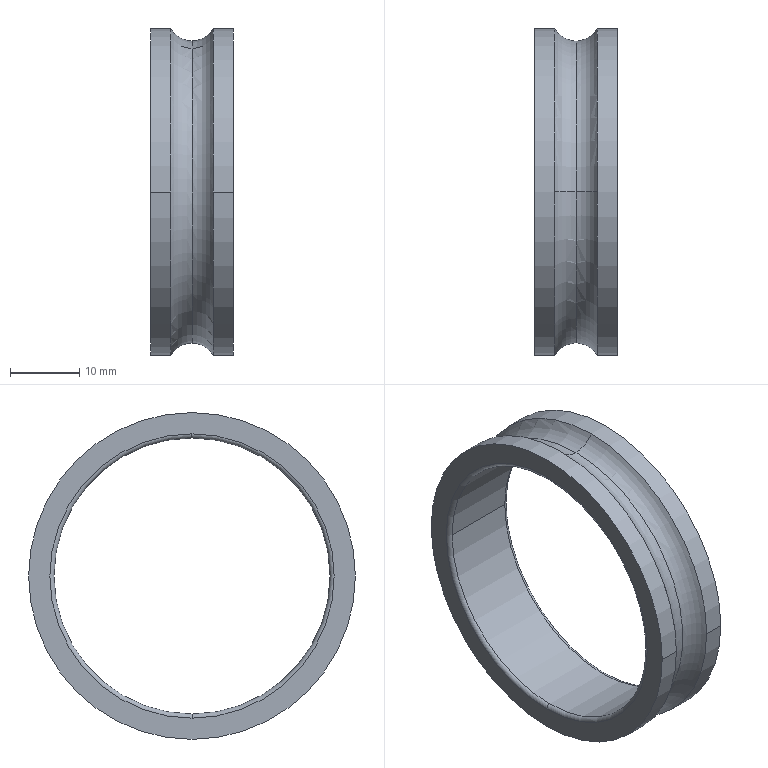Part | STEP file | bearing_6908_01V11 | 1 solid | 16 faces | box 12 x 47.33 x 47.33 mm | volume 4895 mm3 | torus 8 | cylinder 6 | plane 2 | commonest cylinder face diameters 47.33 x4 40 x2
STEP:
#1=CARTESIAN_POINT('',(0.,0.,0.));
#2=DIRECTION('',(0.,0.,1.));
#3=DIRECTION('',(1.,0.,0.));
#4=AXIS2_PLACEMENT_3D('',#1,#2,#3);
#5=CARTESIAN_POINT('',(3.099,0.,-23.665));
#6=VERTEX_POINT('',#5);
#7=CARTESIAN_POINT('',(3.099,23.665,0.));
#8=VERTEX_POINT('',#7);
#9=CARTESIAN_POINT('',(3.099,0.,0.));
#10=DIRECTION('',(1.,0.,0.));
#11=DIRECTION('',(0.,1.,0.));
#12=AXIS2_PLACEMENT_3D('',#9,#10,#11);
#13=CIRCLE('',#12,23.665);
#14=CARTESIAN_POINT('',(0.,0.,0.));
#15=DIRECTION('',(1.,0.,0.));
#16=DIRECTION('',(0.,0.,-1.));
#17=AXIS2_PLACEMENT_3D('',#14,#15,#16);
#18=TOROIDAL_SURFACE('',#17,25.497,3.6);
#19=CARTESIAN_POINT('',(-4.712,2.105));
#20=DIRECTION('',(1.,0.));
#21=VECTOR('',#20,1.);
#22=LINE('',#19,#21);
#23=(GEOMETRIC_REPRESENTATION_CONTEXT(2)PARAMETRIC_REPRESENTATION_CONTEXT()REPRESENTATION_CONTEXT('',''));
#24=DEFINITIONAL_REPRESENTATION('',(#22),#23);
#25=PCURVE('',#18,#24);
#26=CARTESIAN_POINT('',(4.549,0.,0.));
#27=DIRECTION('',(-1.,0.,0.));
#28=DIRECTION('',(0.,1.,0.));
#29=AXIS2_PLACEMENT_3D('',#26,#27,#28);
#30=CYLINDRICAL_SURFACE('',#29,23.665);
#31=CARTESIAN_POINT('',(6.283,1.451));
#32=DIRECTION('',(-1.,0.));
#33=VECTOR('',#32,1.);
#34=LINE('',#31,#33);
#35=(GEOMETRIC_REPRESENTATION_CONTEXT(2)PARAMETRIC_REPRESENTATION_CONTEXT()REPRESENTATION_CONTEXT('',''));
#36=DEFINITIONAL_REPRESENTATION('',(#34),#35);
#37=PCURVE('',#30,#36);
#38=SURFACE_CURVE('',#13,(#25,#37),.PCURVE_S1.);
#39=EDGE_CURVE('',#6,#8,#38,.T.);
#40=ORIENTED_EDGE('',*,*,#39,.T.);
#41=CARTESIAN_POINT('',(3.099,0.,23.665));
#42=VERTEX_POINT('',#41);
#43=CARTESIAN_POINT('',(3.099,0.,0.));
#44=DIRECTION('',(1.,0.,0.));
#45=DIRECTION('',(0.,1.,0.));
#46=AXIS2_PLACEMENT_3D('',#43,#44,#45);
#47=CIRCLE('',#46,23.665);
#48=CARTESIAN_POINT('',(1.571,2.105));
#49=DIRECTION('',(1.,0.));
#50=VECTOR('',#49,1.);
#51=LINE('',#48,#50);
#52=(GEOMETRIC_REPRESENTATION_CONTEXT(2)PARAMETRIC_REPRESENTATION_CONTEXT()REPRESENTATION_CONTEXT('',''));
#53=DEFINITIONAL_REPRESENTATION('',(#51),#52);
#54=PCURVE('',#18,#53);
#55=CARTESIAN_POINT('',(4.549,0.,0.));
#56=DIRECTION('',(-1.,0.,0.));
#57=DIRECTION('',(0.,1.,0.));
#58=AXIS2_PLACEMENT_3D('',#55,#56,#57);
#59=CYLINDRICAL_SURFACE('',#58,23.665);
#60=CARTESIAN_POINT('',(6.283,1.451));
#61=DIRECTION('',(-1.,0.));
#62=VECTOR('',#61,1.);
#63=LINE('',#60,#62);
#64=(GEOMETRIC_REPRESENTATION_CONTEXT(2)PARAMETRIC_REPRESENTATION_CONTEXT()REPRESENTATION_CONTEXT('',''));
#65=DEFINITIONAL_REPRESENTATION('',(#63),#64);
#66=PCURVE('',#59,#65);
#67=SURFACE_CURVE('',#47,(#54,#66),.PCURVE_S1.);
#68=EDGE_CURVE('',#8,#42,#67,.T.);
#69=ORIENTED_EDGE('',*,*,#68,.T.);
#70=CARTESIAN_POINT('',(0.,0.,21.898));
#71=VERTEX_POINT('',#70);
#72=CARTESIAN_POINT('',(0.,0.,25.497));
#73=DIRECTION('',(0.,1.,0.));
#74=DIRECTION('',(0.,0.,1.));
#75=AXIS2_PLACEMENT_3D('',#72,#73,#74);
#76=CIRCLE('',#75,3.6);
#77=CARTESIAN_POINT('',(3.142,0.));
#78=DIRECTION('',(0.,1.));
#79=VECTOR('',#78,1.);
#80=LINE('',#77,#79);
#81=(GEOMETRIC_REPRESENTATION_CONTEXT(2)PARAMETRIC_REPRESENTATION_CONTEXT()REPRESENTATION_CONTEXT('',''));
#82=DEFINITIONAL_REPRESENTATION('',(#80),#81);
#83=PCURVE('',#18,#82);
#84=CARTESIAN_POINT('',(0.,0.,0.));
#85=DIRECTION('',(1.,0.,0.));
#86=DIRECTION('',(0.,0.,-1.));
#87=AXIS2_PLACEMENT_3D('',#84,#85,#86);
#88=TOROIDAL_SURFACE('',#87,25.497,3.6);
#89=CARTESIAN_POINT('',(3.142,0.));
#90=DIRECTION('',(0.,1.));
#91=VECTOR('',#90,1.);
#92=LINE('',#89,#91);
#93=(GEOMETRIC_REPRESENTATION_CONTEXT(2)PARAMETRIC_REPRESENTATION_CONTEXT()REPRESENTATION_CONTEXT('',''));
#94=DEFINITIONAL_REPRESENTATION('',(#92),#93);
#95=PCURVE('',#88,#94);
#96=SURFACE_CURVE('',#76,(#83,#95),.PCURVE_S1.);
#97=EDGE_CURVE('',#42,#71,#96,.T.);
#98=ORIENTED_EDGE('',*,*,#97,.T.);
#99=CARTESIAN_POINT('',(0.,0.,-21.898));
#100=VERTEX_POINT('',#99);
#101=CARTESIAN_POINT('',(0.,0.,0.));
#102=DIRECTION('',(1.,0.,0.));
#103=DIRECTION('',(0.,0.,-1.));
#104=AXIS2_PLACEMENT_3D('',#101,#102,#103);
#105=CIRCLE('',#104,21.898);
#106=CARTESIAN_POINT('',(0.,3.142));
#107=DIRECTION('',(1.,0.));
#108=VECTOR('',#107,1.);
#109=LINE('',#106,#108);
#110=(GEOMETRIC_REPRESENTATION_CONTEXT(2)PARAMETRIC_REPRESENTATION_CONTEXT()REPRESENTATION_CONTEXT('',''));
#111=DEFINITIONAL_REPRESENTATION('',(#109),#110);
#112=PCURVE('',#18,#111);
#113=CARTESIAN_POINT('',(0.,0.,0.));
#114=DIRECTION('',(1.,0.,0.));
#115=DIRECTION('',(0.,0.,-1.));
#116=AXIS2_PLACEMENT_3D('',#113,#114,#115);
#117=TOROIDAL_SURFACE('',#116,25.497,3.6);
#118=CARTESIAN_POINT('',(0.,3.142));
#119=DIRECTION('',(1.,0.));
#120=VECTOR('',#119,1.);
#121=LINE('',#118,#120);
#122=(GEOMETRIC_REPRESENTATION_CONTEXT(2)PARAMETRIC_REPRESENTATION_CONTEXT()REPRESENTATION_CONTEXT('',''));
#123=DEFINITIONAL_REPRESENTATION('',(#121),#122);
#124=PCURVE('',#117,#123);
#125=SURFACE_CURVE('',#105,(#112,#124),.PCURVE_S1.);
#126=EDGE_CURVE('',#100,#71,#125,.T.);
#127=ORIENTED_EDGE('',*,*,#126,.F.);
#128=CARTESIAN_POINT('',(0.,0.,-25.497));
#129=DIRECTION('',(0.,-1.,0.));
#130=DIRECTION('',(0.,0.,-1.));
#131=AXIS2_PLACEMENT_3D('',#128,#129,#130);
#132=CIRCLE('',#131,3.6);
#133=CARTESIAN_POINT('',(0.,0.));
#134=DIRECTION('',(0.,1.));
#135=VECTOR('',#134,1.);
#136=LINE('',#133,#135);
#137=(GEOMETRIC_REPRESENTATION_CONTEXT(2)PARAMETRIC_REPRESENTATION_CONTEXT()REPRESENTATION_CONTEXT('',''));
#138=DEFINITIONAL_REPRESENTATION('',(#136),#137);
#139=PCURVE('',#18,#138);
#140=CARTESIAN_POINT('',(6.283,0.));
#141=DIRECTION('',(0.,1.));
#142=VECTOR('',#141,1.);
#143=LINE('',#140,#142);
#144=(GEOMETRIC_REPRESENTATION_CONTEXT(2)PARAMETRIC_REPRESENTATION_CONTEXT()REPRESENTATION_CONTEXT('',''));
#145=DEFINITIONAL_REPRESENTATION('',(#143),#144);
#146=PCURVE('',#88,#145);
#147=SURFACE_CURVE('',#132,(#139,#146),.PCURVE_S1.);
#148=EDGE_CURVE('',#6,#100,#147,.T.);
#149=ORIENTED_EDGE('',*,*,#148,.F.);
#150=EDGE_LOOP('',(#40,#69,#98,#127,#149));
#151=FACE_BOUND('',#150,.F.);
#152=ADVANCED_FACE('',(#151),#18,.F.);
#153=CARTESIAN_POINT('',(3.099,-23.665,0.));
#154=VERTEX_POINT('',#153);
#155=CARTESIAN_POINT('',(3.099,0.,0.));
#156=DIRECTION('',(1.,0.,0.));
#157=DIRECTION('',(0.,1.,0.));
#158=AXIS2_PLACEMENT_3D('',#155,#156,#157);
#159=CIRCLE('',#158,23.665);
#160=CARTESIAN_POINT('',(1.571,2.105));
#161=DIRECTION('',(1.,0.));
#162=VECTOR('',#161,1.);
#163=LINE('',#160,#162);
#164=(GEOMETRIC_REPRESENTATION_CONTEXT(2)PARAMETRIC_REPRESENTATION_CONTEXT()REPRESENTATION_CONTEXT('',''));
#165=DEFINITIONAL_REPRESENTATION('',(#163),#164);
#166=PCURVE('',#88,#165);
#167=CARTESIAN_POINT('',(6.283,1.451));
#168=DIRECTION('',(-1.,0.));
#169=VECTOR('',#168,1.);
#170=LINE('',#167,#169);
#171=(GEOMETRIC_REPRESENTATION_CONTEXT(2)PARAMETRIC_REPRESENTATION_CONTEXT()REPRESENTATION_CONTEXT('',''));
#172=DEFINITIONAL_REPRESENTATION('',(#170),#171);
#173=PCURVE('',#59,#172);
#174=SURFACE_CURVE('',#159,(#166,#173),.PCURVE_S1.);
#175=EDGE_CURVE('',#42,#154,#174,.T.);
#176=ORIENTED_EDGE('',*,*,#175,.T.);
#177=CARTESIAN_POINT('',(3.099,0.,0.));
#178=DIRECTION('',(1.,0.,0.));
#179=DIRECTION('',(0.,1.,0.));
#180=AXIS2_PLACEMENT_3D('',#177,#178,#179);
#181=CIRCLE('',#180,23.665);
#182=CARTESIAN_POINT('',(1.571,2.105));
#183=DIRECTION('',(1.,0.));
#184=VECTOR('',#183,1.);
#185=LINE('',#182,#184);
#186=(GEOMETRIC_REPRESENTATION_CONTEXT(2)PARAMETRIC_REPRESENTATION_CONTEXT()REPRESENTATION_CONTEXT('',''));
#187=DEFINITIONAL_REPRESENTATION('',(#185),#186);
#188=PCURVE('',#88,#187);
#189=CARTESIAN_POINT('',(6.283,1.451));
#190=DIRECTION('',(-1.,0.));
#191=VECTOR('',#190,1.);
#192=LINE('',#189,#191);
#193=(GEOMETRIC_REPRESENTATION_CONTEXT(2)PARAMETRIC_REPRESENTATION_CONTEXT()REPRESENTATION_CONTEXT('',''));
#194=DEFINITIONAL_REPRESENTATION('',(#192),#193);
#195=PCURVE('',#30,#194);
#196=SURFACE_CURVE('',#181,(#188,#195),.PCURVE_S1.);
#197=EDGE_CURVE('',#154,#6,#196,.T.);
#198=ORIENTED_EDGE('',*,*,#197,.T.);
#199=ORIENTED_EDGE('',*,*,#148,.T.);
#200=CARTESIAN_POINT('',(0.,0.,0.));
#201=DIRECTION('',(1.,0.,0.));
#202=DIRECTION('',(0.,0.,-1.));
#203=AXIS2_PLACEMENT_3D('',#200,#201,#202);
#204=CIRCLE('',#203,21.898);
#205=CARTESIAN_POINT('',(0.,3.142));
#206=DIRECTION('',(1.,0.));
#207=VECTOR('',#206,1.);
#208=LINE('',#205,#207);
#209=(GEOMETRIC_REPRESENTATION_CONTEXT(2)PARAMETRIC_REPRESENTATION_CONTEXT()REPRESENTATION_CONTEXT('',''));
#210=DEFINITIONAL_REPRESENTATION('',(#208),#209);
#211=PCURVE('',#88,#210);
#212=CARTESIAN_POINT('',(0.,0.,0.));
#213=DIRECTION('',(1.,0.,0.));
#214=DIRECTION('',(0.,0.,-1.));
#215=AXIS2_PLACEMENT_3D('',#212,#213,#214);
#216=TOROIDAL_SURFACE('',#215,25.497,3.6);
#217=CARTESIAN_POINT('',(0.,3.142));
#218=DIRECTION('',(1.,0.));
#219=VECTOR('',#218,1.);
#220=LINE('',#217,#219);
#221=(GEOMETRIC_REPRESENTATION_CONTEXT(2)PARAMETRIC_REPRESENTATION_CONTEXT()REPRESENTATION_CONTEXT('',''));
#222=DEFINITIONAL_REPRESENTATION('',(#220),#221);
#223=PCURVE('',#216,#222);
#224=SURFACE_CURVE('',#204,(#211,#223),.PCURVE_S1.);
#225=EDGE_CURVE('',#71,#100,#224,.T.);
#226=ORIENTED_EDGE('',*,*,#225,.F.);
#227=ORIENTED_EDGE('',*,*,#97,.F.);
#228=EDGE_LOOP('',(#176,#198,#199,#226,#227));
#229=FACE_BOUND('',#228,.F.);
#230=ADVANCED_FACE('',(#229),#88,.F.);
#231=CARTESIAN_POINT('',(-3.099,-23.665,0.));
#232=VERTEX_POINT('',#231);
#233=CARTESIAN_POINT('',(-3.099,0.,-23.665));
#234=VERTEX_POINT('',#233);
#235=CARTESIAN_POINT('',(-3.099,0.,0.));
#236=DIRECTION('',(1.,0.,0.));
#237=DIRECTION('',(0.,1.,0.));
#238=AXIS2_PLACEMENT_3D('',#235,#236,#237);
#239=CIRCLE('',#238,23.665);
#240=CARTESIAN_POINT('',(-4.549,0.,0.));
#241=DIRECTION('',(-1.,0.,0.));
#242=DIRECTION('',(0.,1.,0.));
#243=AXIS2_PLACEMENT_3D('',#240,#241,#242);
#244=CYLINDRICAL_SURFACE('',#243,23.665);
#245=CARTESIAN_POINT('',(6.283,-1.451));
#246=DIRECTION('',(-1.,0.));
#247=VECTOR('',#246,1.);
#248=LINE('',#245,#247);
#249=(GEOMETRIC_REPRESENTATION_CONTEXT(2)PARAMETRIC_REPRESENTATION_CONTEXT()REPRESENTATION_CONTEXT('',''));
#250=DEFINITIONAL_REPRESENTATION('',(#248),#249);
#251=PCURVE('',#244,#250);
#252=CARTESIAN_POINT('',(1.571,4.178));
#253=DIRECTION('',(1.,0.));
#254=VECTOR('',#253,1.);
#255=LINE('',#252,#254);
#256=(GEOMETRIC_REPRESENTATION_CONTEXT(2)PARAMETRIC_REPRESENTATION_CONTEXT()REPRESENTATION_CONTEXT('',''));
#257=DEFINITIONAL_REPRESENTATION('',(#255),#256);
#258=PCURVE('',#216,#257);
#259=SURFACE_CURVE('',#239,(#251,#258),.PCURVE_S1.);
#260=EDGE_CURVE('',#232,#234,#259,.T.);
#261=ORIENTED_EDGE('',*,*,#260,.F.);
#262=CARTESIAN_POINT('',(-6.,-23.665,0.));
#263=VERTEX_POINT('',#262);
#264=CARTESIAN_POINT('',(-4.549,-23.665,0.));
#265=DIRECTION('',(-1.,0.,0.));
#266=VECTOR('',#265,1.);
#267=LINE('',#264,#266);
#268=CARTESIAN_POINT('',(3.142,0.));
#269=DIRECTION('',(0.,1.));
#270=VECTOR('',#269,1.);
#271=LINE('',#268,#270);
#272=(GEOMETRIC_REPRESENTATION_CONTEXT(2)PARAMETRIC_REPRESENTATION_CONTEXT()REPRESENTATION_CONTEXT('',''));
#273=DEFINITIONAL_REPRESENTATION('',(#271),#272);
#274=PCURVE('',#244,#273);
#275=CARTESIAN_POINT('',(-4.549,0.,0.));
#276=DIRECTION('',(-1.,0.,0.));
#277=DIRECTION('',(0.,1.,0.));
#278=AXIS2_PLACEMENT_3D('',#275,#276,#277);
#279=CYLINDRICAL_SURFACE('',#278,23.665);
#280=CARTESIAN_POINT('',(3.142,0.));
#281=DIRECTION('',(0.,1.));
#282=VECTOR('',#281,1.);
#283=LINE('',#280,#282);
#284=(GEOMETRIC_REPRESENTATION_CONTEXT(2)PARAMETRIC_REPRESENTATION_CONTEXT()REPRESENTATION_CONTEXT('',''));
#285=DEFINITIONAL_REPRESENTATION('',(#283),#284);
#286=PCURVE('',#279,#285);
#287=SURFACE_CURVE('',#267,(#274,#286),.PCURVE_S1.);
#288=EDGE_CURVE('',#232,#263,#287,.T.);
#289=ORIENTED_EDGE('',*,*,#288,.T.);
#290=CARTESIAN_POINT('',(-6.,23.665,0.));
#291=VERTEX_POINT('',#290);
#292=CARTESIAN_POINT('',(-6.,0.,0.));
#293=DIRECTION('',(1.,0.,0.));
#294=DIRECTION('',(0.,1.,0.));
#295=AXIS2_PLACEMENT_3D('',#292,#293,#294);
#296=CIRCLE('',#295,23.665);
#297=CARTESIAN_POINT('',(6.283,1.451));
#298=DIRECTION('',(-1.,0.));
#299=VECTOR('',#298,1.);
#300=LINE('',#297,#299);
#301=(GEOMETRIC_REPRESENTATION_CONTEXT(2)PARAMETRIC_REPRESENTATION_CONTEXT()REPRESENTATION_CONTEXT('',''));
#302=DEFINITIONAL_REPRESENTATION('',(#300),#301);
#303=PCURVE('',#244,#302);
#304=CARTESIAN_POINT('',(-6.,22.133,0.));
#305=DIRECTION('',(-1.,0.,0.));
#306=DIRECTION('',(0.,-1.,0.));
#307=AXIS2_PLACEMENT_3D('',#304,#305,#306);
#308=PLANE('',#307);
#309=CARTESIAN_POINT('',(-1.532,0.));
#310=CARTESIAN_POINT('',(-1.532,40.989));
#311=CARTESIAN_POINT('',(33.965,20.494));
#312=CARTESIAN_POINT('',(69.463,0.));
#313=CARTESIAN_POINT('',(33.965,-20.494));
#314=CARTESIAN_POINT('',(-1.532,-40.989));
#315=CARTESIAN_POINT('',(-1.532,0.));
#316=(BOUNDED_CURVE()B_SPLINE_CURVE(2,(#309,#310,#311,#312,#313,#314,#315),.UNSPECIFIED.,.T.,.F.)B_SPLINE_CURVE_WITH_KNOTS((1,2,2,2,2,1),(-2.094,0.,2.094,4.189,6.283,8.378),.UNSPECIFIED.)CURVE()GEOMETRIC_REPRESENTATION_ITEM()RATIONAL_B_SPLINE_CURVE((1.,0.5,1.,0.5,1.,0.5,1.))REPRESENTATION_ITEM(''));
#317=(GEOMETRIC_REPRESENTATION_CONTEXT(2)PARAMETRIC_REPRESENTATION_CONTEXT()REPRESENTATION_CONTEXT('',''));
#318=DEFINITIONAL_REPRESENTATION('',(#316),#317);
#319=PCURVE('',#308,#318);
#320=SURFACE_CURVE('',#296,(#303,#319),.PCURVE_S1.);
#321=EDGE_CURVE('',#263,#291,#320,.T.);
#322=ORIENTED_EDGE('',*,*,#321,.T.);
#323=CARTESIAN_POINT('',(-3.099,23.665,0.));
#324=VERTEX_POINT('',#323);
#325=CARTESIAN_POINT('',(-4.549,23.665,0.));
#326=DIRECTION('',(-1.,0.,0.));
#327=VECTOR('',#326,1.);
#328=LINE('',#325,#327);
#329=CARTESIAN_POINT('',(0.,0.));
#330=DIRECTION('',(0.,1.));
#331=VECTOR('',#330,1.);
#332=LINE('',#329,#331);
#333=(GEOMETRIC_REPRESENTATION_CONTEXT(2)PARAMETRIC_REPRESENTATION_CONTEXT()REPRESENTATION_CONTEXT('',''));
#334=DEFINITIONAL_REPRESENTATION('',(#332),#333);
#335=PCURVE('',#244,#334);
#336=CARTESIAN_POINT('',(6.283,0.));
#337=DIRECTION('',(0.,1.));
#338=VECTOR('',#337,1.);
#339=LINE('',#336,#338);
#340=(GEOMETRIC_REPRESENTATION_CONTEXT(2)PARAMETRIC_REPRESENTATION_CONTEXT()REPRESENTATION_CONTEXT('',''));
#341=DEFINITIONAL_REPRESENTATION('',(#339),#340);
#342=PCURVE('',#279,#341);
#343=SURFACE_CURVE('',#328,(#335,#342),.PCURVE_S1.);
#344=EDGE_CURVE('',#324,#291,#343,.T.);
#345=ORIENTED_EDGE('',*,*,#344,.F.);
#346=CARTESIAN_POINT('',(-3.099,0.,0.));
#347=DIRECTION('',(1.,0.,0.));
#348=DIRECTION('',(0.,1.,0.));
#349=AXIS2_PLACEMENT_3D('',#346,#347,#348);
#350=CIRCLE('',#349,23.665);
#351=CARTESIAN_POINT('',(6.283,-1.451));
#352=DIRECTION('',(-1.,0.));
#353=VECTOR('',#352,1.);
#354=LINE('',#351,#353);
#355=(GEOMETRIC_REPRESENTATION_CONTEXT(2)PARAMETRIC_REPRESENTATION_CONTEXT()REPRESENTATION_CONTEXT('',''));
#356=DEFINITIONAL_REPRESENTATION('',(#354),#355);
#357=PCURVE('',#244,#356);
#358=CARTESIAN_POINT('',(-4.712,4.178));
#359=DIRECTION('',(1.,0.));
#360=VECTOR('',#359,1.);
#361=LINE('',#358,#360);
#362=(GEOMETRIC_REPRESENTATION_CONTEXT(2)PARAMETRIC_REPRESENTATION_CONTEXT()REPRESENTATION_CONTEXT('',''));
#363=DEFINITIONAL_REPRESENTATION('',(#361),#362);
#364=PCURVE('',#117,#363);
#365=SURFACE_CURVE('',#350,(#357,#364),.PCURVE_S1.);
#366=EDGE_CURVE('',#234,#324,#365,.T.);
#367=ORIENTED_EDGE('',*,*,#366,.F.);
#368=EDGE_LOOP('',(#261,#289,#322,#345,#367));
#369=FACE_BOUND('',#368,.T.);
#370=ADVANCED_FACE('',(#369),#244,.T.);
#371=CARTESIAN_POINT('',(0.,0.,-25.497));
#372=DIRECTION('',(0.,-1.,0.));
#373=DIRECTION('',(0.,0.,-1.));
#374=AXIS2_PLACEMENT_3D('',#371,#372,#373);
#375=CIRCLE('',#374,3.6);
#376=CARTESIAN_POINT('',(6.283,0.));
#377=DIRECTION('',(0.,1.));
#378=VECTOR('',#377,1.);
#379=LINE('',#376,#378);
#380=(GEOMETRIC_REPRESENTATION_CONTEXT(2)PARAMETRIC_REPRESENTATION_CONTEXT()REPRESENTATION_CONTEXT('',''));
#381=DEFINITIONAL_REPRESENTATION('',(#379),#380);
#382=PCURVE('',#216,#381);
#383=CARTESIAN_POINT('',(0.,0.));
#384=DIRECTION('',(0.,1.));
#385=VECTOR('',#384,1.);
#386=LINE('',#383,#385);
#387=(GEOMETRIC_REPRESENTATION_CONTEXT(2)PARAMETRIC_REPRESENTATION_CONTEXT()REPRESENTATION_CONTEXT('',''));
#388=DEFINITIONAL_REPRESENTATION('',(#386),#387);
#389=PCURVE('',#117,#388);
#390=SURFACE_CURVE('',#375,(#382,#389),.PCURVE_S1.);
#391=EDGE_CURVE('',#100,#234,#390,.T.);
#392=ORIENTED_EDGE('',*,*,#391,.T.);
#393=ORIENTED_EDGE('',*,*,#260,.F.);
#394=CARTESIAN_POINT('',(-3.099,0.,23.665));
#395=VERTEX_POINT('',#394);
#396=CARTESIAN_POINT('',(-3.099,0.,0.));
#397=DIRECTION('',(1.,0.,0.));
#398=DIRECTION('',(0.,1.,0.));
#399=AXIS2_PLACEMENT_3D('',#396,#397,#398);
#400=CIRCLE('',#399,23.665);
#401=CARTESIAN_POINT('',(1.571,4.178));
#402=DIRECTION('',(1.,0.));
#403=VECTOR('',#402,1.);
#404=LINE('',#401,#403);
#405=(GEOMETRIC_REPRESENTATION_CONTEXT(2)PARAMETRIC_REPRESENTATION_CONTEXT()REPRESENTATION_CONTEXT('',''));
#406=DEFINITIONAL_REPRESENTATION('',(#404),#405);
#407=PCURVE('',#216,#406);
#408=CARTESIAN_POINT('',(6.283,-1.451));
#409=DIRECTION('',(-1.,0.));
#410=VECTOR('',#409,1.);
#411=LINE('',#408,#410);
#412=(GEOMETRIC_REPRESENTATION_CONTEXT(2)PARAMETRIC_REPRESENTATION_CONTEXT()REPRESENTATION_CONTEXT('',''));
#413=DEFINITIONAL_REPRESENTATION('',(#411),#412);
#414=PCURVE('',#279,#413);
#415=SURFACE_CURVE('',#400,(#407,#414),.PCURVE_S1.);
#416=EDGE_CURVE('',#395,#232,#415,.T.);
#417=ORIENTED_EDGE('',*,*,#416,.F.);
#418=CARTESIAN_POINT('',(0.,0.,25.497));
#419=DIRECTION('',(0.,1.,0.));
#420=DIRECTION('',(0.,0.,1.));
#421=AXIS2_PLACEMENT_3D('',#418,#419,#420);
#422=CIRCLE('',#421,3.6);
#423=CARTESIAN_POINT('',(3.142,0.));
#424=DIRECTION('',(0.,1.));
#425=VECTOR('',#424,1.);
#426=LINE('',#423,#425);
#427=(GEOMETRIC_REPRESENTATION_CONTEXT(2)PARAMETRIC_REPRESENTATION_CONTEXT()REPRESENTATION_CONTEXT('',''));
#428=DEFINITIONAL_REPRESENTATION('',(#426),#427);
#429=PCURVE('',#216,#428);
#430=CARTESIAN_POINT('',(3.142,0.));
#431=DIRECTION('',(0.,1.));
#432=VECTOR('',#431,1.);
#433=LINE('',#430,#432);
#434=(GEOMETRIC_REPRESENTATION_CONTEXT(2)PARAMETRIC_REPRESENTATION_CONTEXT()REPRESENTATION_CONTEXT('',''));
#435=DEFINITIONAL_REPRESENTATION('',(#433),#434);
#436=PCURVE('',#117,#435);
#437=SURFACE_CURVE('',#422,(#429,#436),.PCURVE_S1.);
#438=EDGE_CURVE('',#71,#395,#437,.T.);
#439=ORIENTED_EDGE('',*,*,#438,.F.);
#440=ORIENTED_EDGE('',*,*,#225,.T.);
#441=EDGE_LOOP('',(#392,#393,#417,#439,#440));
#442=FACE_BOUND('',#441,.F.);
#443=ADVANCED_FACE('',(#442),#216,.F.);
#444=CARTESIAN_POINT('',(6.,-23.665,0.));
#445=VERTEX_POINT('',#444);
#446=CARTESIAN_POINT('',(6.,23.665,0.));
#447=VERTEX_POINT('',#446);
#448=CARTESIAN_POINT('',(6.,0.,0.));
#449=DIRECTION('',(1.,0.,0.));
#450=DIRECTION('',(0.,1.,0.));
#451=AXIS2_PLACEMENT_3D('',#448,#449,#450);
#452=CIRCLE('',#451,23.665);
#453=CARTESIAN_POINT('',(6.283,-1.451));
#454=DIRECTION('',(-1.,0.));
#455=VECTOR('',#454,1.);
#456=LINE('',#453,#455);
#457=(GEOMETRIC_REPRESENTATION_CONTEXT(2)PARAMETRIC_REPRESENTATION_CONTEXT()REPRESENTATION_CONTEXT('',''));
#458=DEFINITIONAL_REPRESENTATION('',(#456),#457);
#459=PCURVE('',#30,#458);
#460=CARTESIAN_POINT('',(6.,22.133,0.));
#461=DIRECTION('',(1.,0.,0.));
#462=DIRECTION('',(0.,1.,0.));
#463=AXIS2_PLACEMENT_3D('',#460,#461,#462);
#464=PLANE('',#463);
#465=CARTESIAN_POINT('',(-22.133,0.));
#466=DIRECTION('',(1.,0.));
#467=AXIS2_PLACEMENT_2D('',#465,#466);
#468=CIRCLE('',#467,23.665);
#469=(GEOMETRIC_REPRESENTATION_CONTEXT(2)PARAMETRIC_REPRESENTATION_CONTEXT()REPRESENTATION_CONTEXT('',''));
#470=DEFINITIONAL_REPRESENTATION('',(#468),#469);
#471=PCURVE('',#464,#470);
#472=SURFACE_CURVE('',#452,(#459,#471),.PCURVE_S1.);
#473=EDGE_CURVE('',#445,#447,#472,.T.);
#474=ORIENTED_EDGE('',*,*,#473,.F.);
#475=CARTESIAN_POINT('',(4.549,-23.665,0.));
#476=DIRECTION('',(-1.,0.,0.));
#477=VECTOR('',#476,1.);
#478=LINE('',#475,#477);
#479=CARTESIAN_POINT('',(3.142,0.));
#480=DIRECTION('',(0.,1.));
#481=VECTOR('',#480,1.);
#482=LINE('',#479,#481);
#483=(GEOMETRIC_REPRESENTATION_CONTEXT(2)PARAMETRIC_REPRESENTATION_CONTEXT()REPRESENTATION_CONTEXT('',''));
#484=DEFINITIONAL_REPRESENTATION('',(#482),#483);
#485=PCURVE('',#30,#484);
#486=CARTESIAN_POINT('',(3.142,0.));
#487=DIRECTION('',(0.,1.));
#488=VECTOR('',#487,1.);
#489=LINE('',#486,#488);
#490=(GEOMETRIC_REPRESENTATION_CONTEXT(2)PARAMETRIC_REPRESENTATION_CONTEXT()REPRESENTATION_CONTEXT('',''));
#491=DEFINITIONAL_REPRESENTATION('',(#489),#490);
#492=PCURVE('',#59,#491);
#493=SURFACE_CURVE('',#478,(#485,#492),.PCURVE_S1.);
#494=EDGE_CURVE('',#445,#154,#493,.T.);
#495=ORIENTED_EDGE('',*,*,#494,.T.);
#496=ORIENTED_EDGE('',*,*,#197,.T.);
#497=ORIENTED_EDGE('',*,*,#39,.T.);
#498=CARTESIAN_POINT('',(4.549,23.665,0.));
#499=DIRECTION('',(-1.,0.,0.));
#500=VECTOR('',#499,1.);
#501=LINE('',#498,#500);
#502=CARTESIAN_POINT('',(0.,0.));
#503=DIRECTION('',(0.,1.));
#504=VECTOR('',#503,1.);
#505=LINE('',#502,#504);
#506=(GEOMETRIC_REPRESENTATION_CONTEXT(2)PARAMETRIC_REPRESENTATION_CONTEXT()REPRESENTATION_CONTEXT('',''));
#507=DEFINITIONAL_REPRESENTATION('',(#505),#506);
#508=PCURVE('',#30,#507);
#509=CARTESIAN_POINT('',(6.283,0.));
#510=DIRECTION('',(0.,1.));
#511=VECTOR('',#510,1.);
#512=LINE('',#509,#511);
#513=(GEOMETRIC_REPRESENTATION_CONTEXT(2)PARAMETRIC_REPRESENTATION_CONTEXT()REPRESENTATION_CONTEXT('',''));
#514=DEFINITIONAL_REPRESENTATION('',(#512),#513);
#515=PCURVE('',#59,#514);
#516=SURFACE_CURVE('',#501,(#508,#515),.PCURVE_S1.);
#517=EDGE_CURVE('',#447,#8,#516,.T.);
#518=ORIENTED_EDGE('',*,*,#517,.F.);
#519=EDGE_LOOP('',(#474,#495,#496,#497,#518));
#520=FACE_BOUND('',#519,.T.);
#521=ADVANCED_FACE('',(#520),#30,.T.);
#522=CARTESIAN_POINT('',(6.,0.,-20.6));
#523=VERTEX_POINT('',#522);
#524=CARTESIAN_POINT('',(6.,0.,20.6));
#525=VERTEX_POINT('',#524);
#526=CARTESIAN_POINT('',(6.,0.,0.));
#527=DIRECTION('',(1.,0.,0.));
#528=DIRECTION('',(0.,1.,0.));
#529=AXIS2_PLACEMENT_3D('',#526,#527,#528);
#530=CIRCLE('',#529,20.6);
#531=CARTESIAN_POINT('',(5.4,0.,0.));
#532=DIRECTION('',(1.,0.,0.));
#533=DIRECTION('',(0.,0.,-1.));
#534=AXIS2_PLACEMENT_3D('',#531,#532,#533);
#535=TOROIDAL_SURFACE('',#534,20.6,0.6);
#536=CARTESIAN_POINT('',(-4.712,1.571));
#537=DIRECTION('',(1.,0.));
#538=VECTOR('',#537,1.);
#539=LINE('',#536,#538);
#540=(GEOMETRIC_REPRESENTATION_CONTEXT(2)PARAMETRIC_REPRESENTATION_CONTEXT()REPRESENTATION_CONTEXT('',''));
#541=DEFINITIONAL_REPRESENTATION('',(#539),#540);
#542=PCURVE('',#535,#541);
#543=CARTESIAN_POINT('',(-22.133,0.));
#544=DIRECTION('',(1.,0.));
#545=AXIS2_PLACEMENT_2D('',#543,#544);
#546=CIRCLE('',#545,20.6);
#547=(GEOMETRIC_REPRESENTATION_CONTEXT(2)PARAMETRIC_REPRESENTATION_CONTEXT()REPRESENTATION_CONTEXT('',''));
#548=DEFINITIONAL_REPRESENTATION('',(#546),#547);
#549=PCURVE('',#464,#548);
#550=SURFACE_CURVE('',#530,(#542,#549),.PCURVE_S1.);
#551=EDGE_CURVE('',#523,#525,#550,.T.);
#552=ORIENTED_EDGE('',*,*,#551,.T.);
#553=CARTESIAN_POINT('',(5.4,0.,20.));
#554=VERTEX_POINT('',#553);
#555=CARTESIAN_POINT('',(5.4,0.,20.6));
#556=DIRECTION('',(0.,1.,0.));
#557=DIRECTION('',(0.,0.,1.));
#558=AXIS2_PLACEMENT_3D('',#555,#556,#557);
#559=CIRCLE('',#558,0.6);
#560=CARTESIAN_POINT('',(3.142,0.));
#561=DIRECTION('',(0.,1.));
#562=VECTOR('',#561,1.);
#563=LINE('',#560,#562);
#564=(GEOMETRIC_REPRESENTATION_CONTEXT(2)PARAMETRIC_REPRESENTATION_CONTEXT()REPRESENTATION_CONTEXT('',''));
#565=DEFINITIONAL_REPRESENTATION('',(#563),#564);
#566=PCURVE('',#535,#565);
#567=CARTESIAN_POINT('',(5.4,0.,0.));
#568=DIRECTION('',(1.,0.,0.));
#569=DIRECTION('',(0.,0.,-1.));
#570=AXIS2_PLACEMENT_3D('',#567,#568,#569);
#571=TOROIDAL_SURFACE('',#570,20.6,0.6);
#572=CARTESIAN_POINT('',(3.142,0.));
#573=DIRECTION('',(0.,1.));
#574=VECTOR('',#573,1.);
#575=LINE('',#572,#574);
#576=(GEOMETRIC_REPRESENTATION_CONTEXT(2)PARAMETRIC_REPRESENTATION_CONTEXT()REPRESENTATION_CONTEXT('',''));
#577=DEFINITIONAL_REPRESENTATION('',(#575),#576);
#578=PCURVE('',#571,#577);
#579=SURFACE_CURVE('',#559,(#566,#578),.PCURVE_S1.);
#580=EDGE_CURVE('',#525,#554,#579,.T.);
#581=ORIENTED_EDGE('',*,*,#580,.T.);
#582=CARTESIAN_POINT('',(5.4,20.,0.));
#583=VERTEX_POINT('',#582);
#584=CARTESIAN_POINT('',(5.4,0.,0.));
#585=DIRECTION('',(1.,0.,0.));
#586=DIRECTION('',(0.,1.,0.));
#587=AXIS2_PLACEMENT_3D('',#584,#585,#586);
#588=CIRCLE('',#587,20.);
#589=CARTESIAN_POINT('',(1.571,3.142));
#590=DIRECTION('',(1.,0.));
#591=VECTOR('',#590,1.);
#592=LINE('',#589,#591);
#593=(GEOMETRIC_REPRESENTATION_CONTEXT(2)PARAMETRIC_REPRESENTATION_CONTEXT()REPRESENTATION_CONTEXT('',''));
#594=DEFINITIONAL_REPRESENTATION('',(#592),#593);
#595=PCURVE('',#535,#594);
#596=CARTESIAN_POINT('',(0.,0.,0.));
#597=DIRECTION('',(-1.,0.,0.));
#598=DIRECTION('',(0.,1.,0.));
#599=AXIS2_PLACEMENT_3D('',#596,#597,#598);
#600=CYLINDRICAL_SURFACE('',#599,20.);
#601=CARTESIAN_POINT('',(6.283,-5.4));
#602=DIRECTION('',(-1.,0.));
#603=VECTOR('',#602,1.);
#604=LINE('',#601,#603);
#605=(GEOMETRIC_REPRESENTATION_CONTEXT(2)PARAMETRIC_REPRESENTATION_CONTEXT()REPRESENTATION_CONTEXT('',''));
#606=DEFINITIONAL_REPRESENTATION('',(#604),#605);
#607=PCURVE('',#600,#606);
#608=SURFACE_CURVE('',#588,(#595,#607),.PCURVE_S1.);
#609=EDGE_CURVE('',#583,#554,#608,.T.);
#610=ORIENTED_EDGE('',*,*,#609,.F.);
#611=CARTESIAN_POINT('',(5.4,0.,-20.));
#612=VERTEX_POINT('',#611);
#613=CARTESIAN_POINT('',(5.4,0.,0.));
#614=DIRECTION('',(1.,0.,0.));
#615=DIRECTION('',(0.,1.,0.));
#616=AXIS2_PLACEMENT_3D('',#613,#614,#615);
#617=CIRCLE('',#616,20.);
#618=CARTESIAN_POINT('',(-4.712,3.142));
#619=DIRECTION('',(1.,0.));
#620=VECTOR('',#619,1.);
#621=LINE('',#618,#620);
#622=(GEOMETRIC_REPRESENTATION_CONTEXT(2)PARAMETRIC_REPRESENTATION_CONTEXT()REPRESENTATION_CONTEXT('',''));
#623=DEFINITIONAL_REPRESENTATION('',(#621),#622);
#624=PCURVE('',#535,#623);
#625=CARTESIAN_POINT('',(0.,0.,0.));
#626=DIRECTION('',(-1.,0.,0.));
#627=DIRECTION('',(0.,1.,0.));
#628=AXIS2_PLACEMENT_3D('',#625,#626,#627);
#629=CYLINDRICAL_SURFACE('',#628,20.);
#630=CARTESIAN_POINT('',(6.283,-5.4));
#631=DIRECTION('',(-1.,0.));
#632=VECTOR('',#631,1.);
#633=LINE('',#630,#632);
#634=(GEOMETRIC_REPRESENTATION_CONTEXT(2)PARAMETRIC_REPRESENTATION_CONTEXT()REPRESENTATION_CONTEXT('',''));
#635=DEFINITIONAL_REPRESENTATION('',(#633),#634);
#636=PCURVE('',#629,#635);
#637=SURFACE_CURVE('',#617,(#624,#636),.PCURVE_S1.);
#638=EDGE_CURVE('',#612,#583,#637,.T.);
#639=ORIENTED_EDGE('',*,*,#638,.F.);
#640=CARTESIAN_POINT('',(5.4,0.,-20.6));
#641=DIRECTION('',(0.,-1.,0.));
#642=DIRECTION('',(0.,0.,-1.));
#643=AXIS2_PLACEMENT_3D('',#640,#641,#642);
#644=CIRCLE('',#643,0.6);
#645=CARTESIAN_POINT('',(0.,0.));
#646=DIRECTION('',(0.,1.));
#647=VECTOR('',#646,1.);
#648=LINE('',#645,#647);
#649=(GEOMETRIC_REPRESENTATION_CONTEXT(2)PARAMETRIC_REPRESENTATION_CONTEXT()REPRESENTATION_CONTEXT('',''));
#650=DEFINITIONAL_REPRESENTATION('',(#648),#649);
#651=PCURVE('',#535,#650);
#652=CARTESIAN_POINT('',(6.283,0.));
#653=DIRECTION('',(0.,1.));
#654=VECTOR('',#653,1.);
#655=LINE('',#652,#654);
#656=(GEOMETRIC_REPRESENTATION_CONTEXT(2)PARAMETRIC_REPRESENTATION_CONTEXT()REPRESENTATION_CONTEXT('',''));
#657=DEFINITIONAL_REPRESENTATION('',(#655),#656);
#658=PCURVE('',#571,#657);
#659=SURFACE_CURVE('',#644,(#651,#658),.PCURVE_S1.);
#660=EDGE_CURVE('',#523,#612,#659,.T.);
#661=ORIENTED_EDGE('',*,*,#660,.F.);
#662=EDGE_LOOP('',(#552,#581,#610,#639,#661));
#663=FACE_BOUND('',#662,.T.);
#664=ADVANCED_FACE('',(#663),#535,.T.);
#665=CARTESIAN_POINT('',(-5.4,20.,0.));
#666=VERTEX_POINT('',#665);
#667=CARTESIAN_POINT('',(0.,20.,0.));
#668=DIRECTION('',(-1.,0.,0.));
#669=VECTOR('',#668,1.);
#670=LINE('',#667,#669);
#671=CARTESIAN_POINT('',(6.283,0.));
#672=DIRECTION('',(0.,1.));
#673=VECTOR('',#672,1.);
#674=LINE('',#671,#673);
#675=(GEOMETRIC_REPRESENTATION_CONTEXT(2)PARAMETRIC_REPRESENTATION_CONTEXT()REPRESENTATION_CONTEXT('',''));
#676=DEFINITIONAL_REPRESENTATION('',(#674),#675);
#677=PCURVE('',#600,#676);
#678=CARTESIAN_POINT('',(0.,0.));
#679=DIRECTION('',(0.,1.));
#680=VECTOR('',#679,1.);
#681=LINE('',#678,#680);
#682=(GEOMETRIC_REPRESENTATION_CONTEXT(2)PARAMETRIC_REPRESENTATION_CONTEXT()REPRESENTATION_CONTEXT('',''));
#683=DEFINITIONAL_REPRESENTATION('',(#681),#682);
#684=PCURVE('',#629,#683);
#685=SURFACE_CURVE('',#670,(#677,#684),.PCURVE_S1.);
#686=EDGE_CURVE('',#583,#666,#685,.T.);
#687=ORIENTED_EDGE('',*,*,#686,.T.);
#688=CARTESIAN_POINT('',(-5.4,0.,20.));
#689=VERTEX_POINT('',#688);
#690=CARTESIAN_POINT('',(-5.4,0.,0.));
#691=DIRECTION('',(1.,0.,0.));
#692=DIRECTION('',(0.,1.,0.));
#693=AXIS2_PLACEMENT_3D('',#690,#691,#692);
#694=CIRCLE('',#693,20.);
#695=CARTESIAN_POINT('',(6.283,5.4));
#696=DIRECTION('',(-1.,0.));
#697=VECTOR('',#696,1.);
#698=LINE('',#695,#697);
#699=(GEOMETRIC_REPRESENTATION_CONTEXT(2)PARAMETRIC_REPRESENTATION_CONTEXT()REPRESENTATION_CONTEXT('',''));
#700=DEFINITIONAL_REPRESENTATION('',(#698),#699);
#701=PCURVE('',#600,#700);
#702=CARTESIAN_POINT('',(-5.4,0.,0.));
#703=DIRECTION('',(1.,0.,0.));
#704=DIRECTION('',(0.,0.,-1.));
#705=AXIS2_PLACEMENT_3D('',#702,#703,#704);
#706=TOROIDAL_SURFACE('',#705,20.6,0.6);
#707=CARTESIAN_POINT('',(1.571,3.142));
#708=DIRECTION('',(1.,0.));
#709=VECTOR('',#708,1.);
#710=LINE('',#707,#709);
#711=(GEOMETRIC_REPRESENTATION_CONTEXT(2)PARAMETRIC_REPRESENTATION_CONTEXT()REPRESENTATION_CONTEXT('',''));
#712=DEFINITIONAL_REPRESENTATION('',(#710),#711);
#713=PCURVE('',#706,#712);
#714=SURFACE_CURVE('',#694,(#701,#713),.PCURVE_S1.);
#715=EDGE_CURVE('',#666,#689,#714,.T.);
#716=ORIENTED_EDGE('',*,*,#715,.T.);
#717=CARTESIAN_POINT('',(-5.4,-20.,0.));
#718=VERTEX_POINT('',#717);
#719=CARTESIAN_POINT('',(-5.4,0.,0.));
#720=DIRECTION('',(1.,0.,0.));
#721=DIRECTION('',(0.,1.,0.));
#722=AXIS2_PLACEMENT_3D('',#719,#720,#721);
#723=CIRCLE('',#722,20.);
#724=CARTESIAN_POINT('',(6.283,5.4));
#725=DIRECTION('',(-1.,0.));
#726=VECTOR('',#725,1.);
#727=LINE('',#724,#726);
#728=(GEOMETRIC_REPRESENTATION_CONTEXT(2)PARAMETRIC_REPRESENTATION_CONTEXT()REPRESENTATION_CONTEXT('',''));
#729=DEFINITIONAL_REPRESENTATION('',(#727),#728);
#730=PCURVE('',#600,#729);
#731=CARTESIAN_POINT('',(-5.4,0.,0.));
#732=DIRECTION('',(1.,0.,0.));
#733=DIRECTION('',(0.,0.,-1.));
#734=AXIS2_PLACEMENT_3D('',#731,#732,#733);
#735=TOROIDAL_SURFACE('',#734,20.6,0.6);
#736=CARTESIAN_POINT('',(1.571,3.142));
#737=DIRECTION('',(1.,0.));
#738=VECTOR('',#737,1.);
#739=LINE('',#736,#738);
#740=(GEOMETRIC_REPRESENTATION_CONTEXT(2)PARAMETRIC_REPRESENTATION_CONTEXT()REPRESENTATION_CONTEXT('',''));
#741=DEFINITIONAL_REPRESENTATION('',(#739),#740);
#742=PCURVE('',#735,#741);
#743=SURFACE_CURVE('',#723,(#730,#742),.PCURVE_S1.);
#744=EDGE_CURVE('',#689,#718,#743,.T.);
#745=ORIENTED_EDGE('',*,*,#744,.T.);
#746=CARTESIAN_POINT('',(5.4,-20.,0.));
#747=VERTEX_POINT('',#746);
#748=CARTESIAN_POINT('',(0.,-20.,0.));
#749=DIRECTION('',(-1.,0.,0.));
#750=VECTOR('',#749,1.);
#751=LINE('',#748,#750);
#752=CARTESIAN_POINT('',(3.142,0.));
#753=DIRECTION('',(0.,1.));
#754=VECTOR('',#753,1.);
#755=LINE('',#752,#754);
#756=(GEOMETRIC_REPRESENTATION_CONTEXT(2)PARAMETRIC_REPRESENTATION_CONTEXT()REPRESENTATION_CONTEXT('',''));
#757=DEFINITIONAL_REPRESENTATION('',(#755),#756);
#758=PCURVE('',#600,#757);
#759=CARTESIAN_POINT('',(3.142,0.));
#760=DIRECTION('',(0.,1.));
#761=VECTOR('',#760,1.);
#762=LINE('',#759,#761);
#763=(GEOMETRIC_REPRESENTATION_CONTEXT(2)PARAMETRIC_REPRESENTATION_CONTEXT()REPRESENTATION_CONTEXT('',''));
#764=DEFINITIONAL_REPRESENTATION('',(#762),#763);
#765=PCURVE('',#629,#764);
#766=SURFACE_CURVE('',#751,(#758,#765),.PCURVE_S1.);
#767=EDGE_CURVE('',#747,#718,#766,.T.);
#768=ORIENTED_EDGE('',*,*,#767,.F.);
#769=CARTESIAN_POINT('',(5.4,0.,0.));
#770=DIRECTION('',(1.,0.,0.));
#771=DIRECTION('',(0.,1.,0.));
#772=AXIS2_PLACEMENT_3D('',#769,#770,#771);
#773=CIRCLE('',#772,20.);
#774=CARTESIAN_POINT('',(6.283,-5.4));
#775=DIRECTION('',(-1.,0.));
#776=VECTOR('',#775,1.);
#777=LINE('',#774,#776);
#778=(GEOMETRIC_REPRESENTATION_CONTEXT(2)PARAMETRIC_REPRESENTATION_CONTEXT()REPRESENTATION_CONTEXT('',''));
#779=DEFINITIONAL_REPRESENTATION('',(#777),#778);
#780=PCURVE('',#600,#779);
#781=CARTESIAN_POINT('',(1.571,3.142));
#782=DIRECTION('',(1.,0.));
#783=VECTOR('',#782,1.);
#784=LINE('',#781,#783);
#785=(GEOMETRIC_REPRESENTATION_CONTEXT(2)PARAMETRIC_REPRESENTATION_CONTEXT()REPRESENTATION_CONTEXT('',''));
#786=DEFINITIONAL_REPRESENTATION('',(#784),#785);
#787=PCURVE('',#571,#786);
#788=SURFACE_CURVE('',#773,(#780,#787),.PCURVE_S1.);
#789=EDGE_CURVE('',#554,#747,#788,.T.);
#790=ORIENTED_EDGE('',*,*,#789,.F.);
#791=ORIENTED_EDGE('',*,*,#609,.F.);
#792=EDGE_LOOP('',(#687,#716,#745,#768,#790,#791));
#793=FACE_BOUND('',#792,.F.);
#794=ADVANCED_FACE('',(#793),#600,.F.);
#795=CARTESIAN_POINT('',(-5.4,0.,-20.));
#796=VERTEX_POINT('',#795);
#797=CARTESIAN_POINT('',(-5.4,0.,0.));
#798=DIRECTION('',(1.,0.,0.));
#799=DIRECTION('',(0.,1.,0.));
#800=AXIS2_PLACEMENT_3D('',#797,#798,#799);
#801=CIRCLE('',#800,20.);
#802=CARTESIAN_POINT('',(-4.712,3.142));
#803=DIRECTION('',(1.,0.));
#804=VECTOR('',#803,1.);
#805=LINE('',#802,#804);
#806=(GEOMETRIC_REPRESENTATION_CONTEXT(2)PARAMETRIC_REPRESENTATION_CONTEXT()REPRESENTATION_CONTEXT('',''));
#807=DEFINITIONAL_REPRESENTATION('',(#805),#806);
#808=PCURVE('',#706,#807);
#809=CARTESIAN_POINT('',(6.283,5.4));
#810=DIRECTION('',(-1.,0.));
#811=VECTOR('',#810,1.);
#812=LINE('',#809,#811);
#813=(GEOMETRIC_REPRESENTATION_CONTEXT(2)PARAMETRIC_REPRESENTATION_CONTEXT()REPRESENTATION_CONTEXT('',''));
#814=DEFINITIONAL_REPRESENTATION('',(#812),#813);
#815=PCURVE('',#629,#814);
#816=SURFACE_CURVE('',#801,(#808,#815),.PCURVE_S1.);
#817=EDGE_CURVE('',#796,#666,#816,.T.);
#818=ORIENTED_EDGE('',*,*,#817,.T.);
#819=ORIENTED_EDGE('',*,*,#715,.T.);
#820=CARTESIAN_POINT('',(-6.,0.,20.6));
#821=VERTEX_POINT('',#820);
#822=CARTESIAN_POINT('',(-5.4,0.,20.6));
#823=DIRECTION('',(0.,1.,0.));
#824=DIRECTION('',(0.,0.,1.));
#825=AXIS2_PLACEMENT_3D('',#822,#823,#824);
#826=CIRCLE('',#825,0.6);
#827=CARTESIAN_POINT('',(3.142,0.));
#828=DIRECTION('',(0.,1.));
#829=VECTOR('',#828,1.);
#830=LINE('',#827,#829);
#831=(GEOMETRIC_REPRESENTATION_CONTEXT(2)PARAMETRIC_REPRESENTATION_CONTEXT()REPRESENTATION_CONTEXT('',''));
#832=DEFINITIONAL_REPRESENTATION('',(#830),#831);
#833=PCURVE('',#706,#832);
#834=CARTESIAN_POINT('',(3.142,0.));
#835=DIRECTION('',(0.,1.));
#836=VECTOR('',#835,1.);
#837=LINE('',#834,#836);
#838=(GEOMETRIC_REPRESENTATION_CONTEXT(2)PARAMETRIC_REPRESENTATION_CONTEXT()REPRESENTATION_CONTEXT('',''));
#839=DEFINITIONAL_REPRESENTATION('',(#837),#838);
#840=PCURVE('',#735,#839);
#841=SURFACE_CURVE('',#826,(#833,#840),.PCURVE_S1.);
#842=EDGE_CURVE('',#689,#821,#841,.T.);
#843=ORIENTED_EDGE('',*,*,#842,.T.);
#844=CARTESIAN_POINT('',(-6.,0.,-20.6));
#845=VERTEX_POINT('',#844);
#846=CARTESIAN_POINT('',(-6.,0.,0.));
#847=DIRECTION('',(1.,0.,0.));
#848=DIRECTION('',(0.,1.,0.));
#849=AXIS2_PLACEMENT_3D('',#846,#847,#848);
#850=CIRCLE('',#849,20.6);
#851=CARTESIAN_POINT('',(-4.712,4.712));
#852=DIRECTION('',(1.,0.));
#853=VECTOR('',#852,1.);
#854=LINE('',#851,#853);
#855=(GEOMETRIC_REPRESENTATION_CONTEXT(2)PARAMETRIC_REPRESENTATION_CONTEXT()REPRESENTATION_CONTEXT('',''));
#856=DEFINITIONAL_REPRESENTATION('',(#854),#855);
#857=PCURVE('',#706,#856);
#858=CARTESIAN_POINT('',(1.532,0.));
#859=CARTESIAN_POINT('',(1.532,35.68));
#860=CARTESIAN_POINT('',(32.432,17.84));
#861=CARTESIAN_POINT('',(63.333,0.));
#862=CARTESIAN_POINT('',(32.432,-17.84));
#863=CARTESIAN_POINT('',(1.532,-35.68));
#864=CARTESIAN_POINT('',(1.532,0.));
#865=(BOUNDED_CURVE()B_SPLINE_CURVE(2,(#858,#859,#860,#861,#862,#863,#864),.UNSPECIFIED.,.T.,.F.)B_SPLINE_CURVE_WITH_KNOTS((1,2,2,2,2,1),(-2.094,0.,2.094,4.189,6.283,8.378),.UNSPECIFIED.)CURVE()GEOMETRIC_REPRESENTATION_ITEM()RATIONAL_B_SPLINE_CURVE((1.,0.5,1.,0.5,1.,0.5,1.))REPRESENTATION_ITEM(''));
#866=(GEOMETRIC_REPRESENTATION_CONTEXT(2)PARAMETRIC_REPRESENTATION_CONTEXT()REPRESENTATION_CONTEXT('',''));
#867=DEFINITIONAL_REPRESENTATION('',(#865),#866);
#868=PCURVE('',#308,#867);
#869=SURFACE_CURVE('',#850,(#857,#868),.PCURVE_S1.);
#870=EDGE_CURVE('',#845,#821,#869,.T.);
#871=ORIENTED_EDGE('',*,*,#870,.F.);
#872=CARTESIAN_POINT('',(-5.4,0.,-20.6));
#873=DIRECTION('',(0.,-1.,0.));
#874=DIRECTION('',(0.,0.,-1.));
#875=AXIS2_PLACEMENT_3D('',#872,#873,#874);
#876=CIRCLE('',#875,0.6);
#877=CARTESIAN_POINT('',(0.,0.));
#878=DIRECTION('',(0.,1.));
#879=VECTOR('',#878,1.);
#880=LINE('',#877,#879);
#881=(GEOMETRIC_REPRESENTATION_CONTEXT(2)PARAMETRIC_REPRESENTATION_CONTEXT()REPRESENTATION_CONTEXT('',''));
#882=DEFINITIONAL_REPRESENTATION('',(#880),#881);
#883=PCURVE('',#706,#882);
#884=CARTESIAN_POINT('',(6.283,0.));
#885=DIRECTION('',(0.,1.));
#886=VECTOR('',#885,1.);
#887=LINE('',#884,#886);
#888=(GEOMETRIC_REPRESENTATION_CONTEXT(2)PARAMETRIC_REPRESENTATION_CONTEXT()REPRESENTATION_CONTEXT('',''));
#889=DEFINITIONAL_REPRESENTATION('',(#887),#888);
#890=PCURVE('',#735,#889);
#891=SURFACE_CURVE('',#876,(#883,#890),.PCURVE_S1.);
#892=EDGE_CURVE('',#796,#845,#891,.T.);
#893=ORIENTED_EDGE('',*,*,#892,.F.);
#894=EDGE_LOOP('',(#818,#819,#843,#871,#893));
#895=FACE_BOUND('',#894,.T.);
#896=ADVANCED_FACE('',(#895),#706,.T.);
#897=ORIENTED_EDGE('',*,*,#842,.F.);
#898=ORIENTED_EDGE('',*,*,#744,.T.);
#899=CARTESIAN_POINT('',(-5.4,0.,0.));
#900=DIRECTION('',(1.,0.,0.));
#901=DIRECTION('',(0.,1.,0.));
#902=AXIS2_PLACEMENT_3D('',#899,#900,#901);
#903=CIRCLE('',#902,20.);
#904=CARTESIAN_POINT('',(1.571,3.142));
#905=DIRECTION('',(1.,0.));
#906=VECTOR('',#905,1.);
#907=LINE('',#904,#906);
#908=(GEOMETRIC_REPRESENTATION_CONTEXT(2)PARAMETRIC_REPRESENTATION_CONTEXT()REPRESENTATION_CONTEXT('',''));
#909=DEFINITIONAL_REPRESENTATION('',(#907),#908);
#910=PCURVE('',#735,#909);
#911=CARTESIAN_POINT('',(6.283,5.4));
#912=DIRECTION('',(-1.,0.));
#913=VECTOR('',#912,1.);
#914=LINE('',#911,#913);
#915=(GEOMETRIC_REPRESENTATION_CONTEXT(2)PARAMETRIC_REPRESENTATION_CONTEXT()REPRESENTATION_CONTEXT('',''));
#916=DEFINITIONAL_REPRESENTATION('',(#914),#915);
#917=PCURVE('',#629,#916);
#918=SURFACE_CURVE('',#903,(#910,#917),.PCURVE_S1.);
#919=EDGE_CURVE('',#718,#796,#918,.T.);
#920=ORIENTED_EDGE('',*,*,#919,.T.);
#921=ORIENTED_EDGE('',*,*,#892,.T.);
#922=CARTESIAN_POINT('',(-6.,0.,0.));
#923=DIRECTION('',(1.,0.,0.));
#924=DIRECTION('',(0.,1.,0.));
#925=AXIS2_PLACEMENT_3D('',#922,#923,#924);
#926=CIRCLE('',#925,20.6);
#927=CARTESIAN_POINT('',(1.571,4.712));
#928=DIRECTION('',(1.,0.));
#929=VECTOR('',#928,1.);
#930=LINE('',#927,#929);
#931=(GEOMETRIC_REPRESENTATION_CONTEXT(2)PARAMETRIC_REPRESENTATION_CONTEXT()REPRESENTATION_CONTEXT('',''));
#932=DEFINITIONAL_REPRESENTATION('',(#930),#931);
#933=PCURVE('',#735,#932);
#934=CARTESIAN_POINT('',(1.532,0.));
#935=CARTESIAN_POINT('',(1.532,35.68));
#936=CARTESIAN_POINT('',(32.432,17.84));
#937=CARTESIAN_POINT('',(63.333,0.));
#938=CARTESIAN_POINT('',(32.432,-17.84));
#939=CARTESIAN_POINT('',(1.532,-35.68));
#940=CARTESIAN_POINT('',(1.532,0.));
#941=(BOUNDED_CURVE()B_SPLINE_CURVE(2,(#934,#935,#936,#937,#938,#939,#940),.UNSPECIFIED.,.T.,.F.)B_SPLINE_CURVE_WITH_KNOTS((1,2,2,2,2,1),(-2.094,0.,2.094,4.189,6.283,8.378),.UNSPECIFIED.)CURVE()GEOMETRIC_REPRESENTATION_ITEM()RATIONAL_B_SPLINE_CURVE((1.,0.5,1.,0.5,1.,0.5,1.))REPRESENTATION_ITEM(''));
#942=(GEOMETRIC_REPRESENTATION_CONTEXT(2)PARAMETRIC_REPRESENTATION_CONTEXT()REPRESENTATION_CONTEXT('',''));
#943=DEFINITIONAL_REPRESENTATION('',(#941),#942);
#944=PCURVE('',#308,#943);
#945=SURFACE_CURVE('',#926,(#933,#944),.PCURVE_S1.);
#946=EDGE_CURVE('',#821,#845,#945,.T.);
#947=ORIENTED_EDGE('',*,*,#946,.F.);
#948=EDGE_LOOP('',(#897,#898,#920,#921,#947));
#949=FACE_BOUND('',#948,.T.);
#950=ADVANCED_FACE('',(#949),#735,.T.);
#951=ORIENTED_EDGE('',*,*,#919,.T.);
#952=ORIENTED_EDGE('',*,*,#817,.T.);
#953=ORIENTED_EDGE('',*,*,#686,.F.);
#954=ORIENTED_EDGE('',*,*,#638,.F.);
#955=CARTESIAN_POINT('',(5.4,0.,0.));
#956=DIRECTION('',(1.,0.,0.));
#957=DIRECTION('',(0.,1.,0.));
#958=AXIS2_PLACEMENT_3D('',#955,#956,#957);
#959=CIRCLE('',#958,20.);
#960=CARTESIAN_POINT('',(6.283,-5.4));
#961=DIRECTION('',(-1.,0.));
#962=VECTOR('',#961,1.);
#963=LINE('',#960,#962);
#964=(GEOMETRIC_REPRESENTATION_CONTEXT(2)PARAMETRIC_REPRESENTATION_CONTEXT()REPRESENTATION_CONTEXT('',''));
#965=DEFINITIONAL_REPRESENTATION('',(#963),#964);
#966=PCURVE('',#629,#965);
#967=CARTESIAN_POINT('',(1.571,3.142));
#968=DIRECTION('',(1.,0.));
#969=VECTOR('',#968,1.);
#970=LINE('',#967,#969);
#971=(GEOMETRIC_REPRESENTATION_CONTEXT(2)PARAMETRIC_REPRESENTATION_CONTEXT()REPRESENTATION_CONTEXT('',''));
#972=DEFINITIONAL_REPRESENTATION('',(#970),#971);
#973=PCURVE('',#571,#972);
#974=SURFACE_CURVE('',#959,(#966,#973),.PCURVE_S1.);
#975=EDGE_CURVE('',#747,#612,#974,.T.);
#976=ORIENTED_EDGE('',*,*,#975,.F.);
#977=ORIENTED_EDGE('',*,*,#767,.T.);
#978=EDGE_LOOP('',(#951,#952,#953,#954,#976,#977));
#979=FACE_BOUND('',#978,.F.);
#980=ADVANCED_FACE('',(#979),#629,.F.);
#981=ORIENTED_EDGE('',*,*,#580,.F.);
#982=CARTESIAN_POINT('',(6.,0.,0.));
#983=DIRECTION('',(1.,0.,0.));
#984=DIRECTION('',(0.,1.,0.));
#985=AXIS2_PLACEMENT_3D('',#982,#983,#984);
#986=CIRCLE('',#985,20.6);
#987=CARTESIAN_POINT('',(1.571,1.571));
#988=DIRECTION('',(1.,0.));
#989=VECTOR('',#988,1.);
#990=LINE('',#987,#989);
#991=(GEOMETRIC_REPRESENTATION_CONTEXT(2)PARAMETRIC_REPRESENTATION_CONTEXT()REPRESENTATION_CONTEXT('',''));
#992=DEFINITIONAL_REPRESENTATION('',(#990),#991);
#993=PCURVE('',#571,#992);
#994=CARTESIAN_POINT('',(-22.133,0.));
#995=DIRECTION('',(1.,0.));
#996=AXIS2_PLACEMENT_2D('',#994,#995);
#997=CIRCLE('',#996,20.6);
#998=(GEOMETRIC_REPRESENTATION_CONTEXT(2)PARAMETRIC_REPRESENTATION_CONTEXT()REPRESENTATION_CONTEXT('',''));
#999=DEFINITIONAL_REPRESENTATION('',(#997),#998);
#1000=PCURVE('',#464,#999);
#1001=SURFACE_CURVE('',#986,(#993,#1000),.PCURVE_S1.);
#1002=EDGE_CURVE('',#525,#523,#1001,.T.);
#1003=ORIENTED_EDGE('',*,*,#1002,.T.);
#1004=ORIENTED_EDGE('',*,*,#660,.T.);
#1005=ORIENTED_EDGE('',*,*,#975,.F.);
#1006=ORIENTED_EDGE('',*,*,#789,.F.);
#1007=EDGE_LOOP('',(#981,#1003,#1004,#1005,#1006));
#1008=FACE_BOUND('',#1007,.T.);
#1009=ADVANCED_FACE('',(#1008),#571,.T.);
#1010=CARTESIAN_POINT('',(6.,0.,0.));
#1011=DIRECTION('',(1.,0.,0.));
#1012=DIRECTION('',(0.,1.,0.));
#1013=AXIS2_PLACEMENT_3D('',#1010,#1011,#1012);
#1014=CIRCLE('',#1013,23.665);
#1015=CARTESIAN_POINT('',(-22.133,0.));
#1016=DIRECTION('',(1.,0.));
#1017=AXIS2_PLACEMENT_2D('',#1015,#1016);
#1018=CIRCLE('',#1017,23.665);
#1019=(GEOMETRIC_REPRESENTATION_CONTEXT(2)PARAMETRIC_REPRESENTATION_CONTEXT()REPRESENTATION_CONTEXT('',''));
#1020=DEFINITIONAL_REPRESENTATION('',(#1018),#1019);
#1021=PCURVE('',#464,#1020);
#1022=CARTESIAN_POINT('',(6.283,-1.451));
#1023=DIRECTION('',(-1.,0.));
#1024=VECTOR('',#1023,1.);
#1025=LINE('',#1022,#1024);
#1026=(GEOMETRIC_REPRESENTATION_CONTEXT(2)PARAMETRIC_REPRESENTATION_CONTEXT()REPRESENTATION_CONTEXT('',''));
#1027=DEFINITIONAL_REPRESENTATION('',(#1025),#1026);
#1028=PCURVE('',#59,#1027);
#1029=SURFACE_CURVE('',#1014,(#1021,#1028),.PCURVE_S1.);
#1030=EDGE_CURVE('',#447,#445,#1029,.T.);
#1031=ORIENTED_EDGE('',*,*,#1030,.T.);
#1032=ORIENTED_EDGE('',*,*,#473,.T.);
#1033=EDGE_LOOP('',(#1031,#1032));
#1034=FACE_BOUND('',#1033,.T.);
#1035=ORIENTED_EDGE('',*,*,#551,.F.);
#1036=ORIENTED_EDGE('',*,*,#1002,.F.);
#1037=EDGE_LOOP('',(#1035,#1036));
#1038=FACE_BOUND('',#1037,.T.);
#1039=ADVANCED_FACE('',(#1034,#1038),#464,.T.);
#1040=ORIENTED_EDGE('',*,*,#494,.F.);
#1041=ORIENTED_EDGE('',*,*,#1030,.F.);
#1042=ORIENTED_EDGE('',*,*,#517,.T.);
#1043=ORIENTED_EDGE('',*,*,#68,.T.);
#1044=ORIENTED_EDGE('',*,*,#175,.T.);
#1045=EDGE_LOOP('',(#1040,#1041,#1042,#1043,#1044));
#1046=FACE_BOUND('',#1045,.T.);
#1047=ADVANCED_FACE('',(#1046),#59,.T.);
#1048=ORIENTED_EDGE('',*,*,#438,.T.);
#1049=CARTESIAN_POINT('',(-3.099,0.,0.));
#1050=DIRECTION('',(1.,0.,0.));
#1051=DIRECTION('',(0.,1.,0.));
#1052=AXIS2_PLACEMENT_3D('',#1049,#1050,#1051);
#1053=CIRCLE('',#1052,23.665);
#1054=CARTESIAN_POINT('',(1.571,4.178));
#1055=DIRECTION('',(1.,0.));
#1056=VECTOR('',#1055,1.);
#1057=LINE('',#1054,#1056);
#1058=(GEOMETRIC_REPRESENTATION_CONTEXT(2)PARAMETRIC_REPRESENTATION_CONTEXT()REPRESENTATION_CONTEXT('',''));
#1059=DEFINITIONAL_REPRESENTATION('',(#1057),#1058);
#1060=PCURVE('',#117,#1059);
#1061=CARTESIAN_POINT('',(6.283,-1.451));
#1062=DIRECTION('',(-1.,0.));
#1063=VECTOR('',#1062,1.);
#1064=LINE('',#1061,#1063);
#1065=(GEOMETRIC_REPRESENTATION_CONTEXT(2)PARAMETRIC_REPRESENTATION_CONTEXT()REPRESENTATION_CONTEXT('',''));
#1066=DEFINITIONAL_REPRESENTATION('',(#1064),#1065);
#1067=PCURVE('',#279,#1066);
#1068=SURFACE_CURVE('',#1053,(#1060,#1067),.PCURVE_S1.);
#1069=EDGE_CURVE('',#324,#395,#1068,.T.);
#1070=ORIENTED_EDGE('',*,*,#1069,.F.);
#1071=ORIENTED_EDGE('',*,*,#366,.F.);
#1072=ORIENTED_EDGE('',*,*,#391,.F.);
#1073=ORIENTED_EDGE('',*,*,#126,.T.);
#1074=EDGE_LOOP('',(#1048,#1070,#1071,#1072,#1073));
#1075=FACE_BOUND('',#1074,.F.);
#1076=ADVANCED_FACE('',(#1075),#117,.F.);
#1077=ORIENTED_EDGE('',*,*,#288,.F.);
#1078=ORIENTED_EDGE('',*,*,#416,.F.);
#1079=ORIENTED_EDGE('',*,*,#1069,.F.);
#1080=ORIENTED_EDGE('',*,*,#344,.T.);
#1081=CARTESIAN_POINT('',(-6.,0.,0.));
#1082=DIRECTION('',(1.,0.,0.));
#1083=DIRECTION('',(0.,1.,0.));
#1084=AXIS2_PLACEMENT_3D('',#1081,#1082,#1083);
#1085=CIRCLE('',#1084,23.665);
#1086=CARTESIAN_POINT('',(6.283,1.451));
#1087=DIRECTION('',(-1.,0.));
#1088=VECTOR('',#1087,1.);
#1089=LINE('',#1086,#1088);
#1090=(GEOMETRIC_REPRESENTATION_CONTEXT(2)PARAMETRIC_REPRESENTATION_CONTEXT()REPRESENTATION_CONTEXT('',''));
#1091=DEFINITIONAL_REPRESENTATION('',(#1089),#1090);
#1092=PCURVE('',#279,#1091);
#1093=CARTESIAN_POINT('',(-1.532,0.));
#1094=CARTESIAN_POINT('',(-1.532,40.989));
#1095=CARTESIAN_POINT('',(33.965,20.494));
#1096=CARTESIAN_POINT('',(69.463,0.));
#1097=CARTESIAN_POINT('',(33.965,-20.494));
#1098=CARTESIAN_POINT('',(-1.532,-40.989));
#1099=CARTESIAN_POINT('',(-1.532,0.));
#1100=(BOUNDED_CURVE()B_SPLINE_CURVE(2,(#1093,#1094,#1095,#1096,#1097,#1098,#1099),.UNSPECIFIED.,.T.,.F.)B_SPLINE_CURVE_WITH_KNOTS((1,2,2,2,2,1),(-2.094,0.,2.094,4.189,6.283,8.378),.UNSPECIFIED.)CURVE()GEOMETRIC_REPRESENTATION_ITEM()RATIONAL_B_SPLINE_CURVE((1.,0.5,1.,0.5,1.,0.5,1.))REPRESENTATION_ITEM(''));
#1101=(GEOMETRIC_REPRESENTATION_CONTEXT(2)PARAMETRIC_REPRESENTATION_CONTEXT()REPRESENTATION_CONTEXT('',''));
#1102=DEFINITIONAL_REPRESENTATION('',(#1100),#1101);
#1103=PCURVE('',#308,#1102);
#1104=SURFACE_CURVE('',#1085,(#1092,#1103),.PCURVE_S1.);
#1105=EDGE_CURVE('',#291,#263,#1104,.T.);
#1106=ORIENTED_EDGE('',*,*,#1105,.T.);
#1107=EDGE_LOOP('',(#1077,#1078,#1079,#1080,#1106));
#1108=FACE_BOUND('',#1107,.T.);
#1109=ADVANCED_FACE('',(#1108),#279,.T.);
#1110=ORIENTED_EDGE('',*,*,#870,.T.);
#1111=ORIENTED_EDGE('',*,*,#946,.T.);
#1112=EDGE_LOOP('',(#1110,#1111));
#1113=FACE_BOUND('',#1112,.T.);
#1114=ORIENTED_EDGE('',*,*,#1105,.F.);
#1115=ORIENTED_EDGE('',*,*,#321,.F.);
#1116=EDGE_LOOP('',(#1114,#1115));
#1117=FACE_BOUND('',#1116,.T.);
#1118=ADVANCED_FACE('',(#1113,#1117),#308,.T.);
#1119=CLOSED_SHELL('',(#152,#230,#370,#443,#521,#664,#794,#896,#950,#980,#1009,#1039,#1047,#1076,#1109,#1118));
#1120=MANIFOLD_SOLID_BREP('',#1119);
#1121=(LENGTH_UNIT()NAMED_UNIT(*)SI_UNIT(.MILLI.,.METRE.));
#1122=UNCERTAINTY_MEASURE_WITH_UNIT(LENGTH_MEASURE(0.0000001),#1121,'','');
#1123=(NAMED_UNIT(*)PLANE_ANGLE_UNIT()SI_UNIT($,.RADIAN.));
#1124=(NAMED_UNIT(*)SI_UNIT($,.STERADIAN.)SOLID_ANGLE_UNIT());
#1125=(GEOMETRIC_REPRESENTATION_CONTEXT(3)GLOBAL_UNCERTAINTY_ASSIGNED_CONTEXT((#1122))GLOBAL_UNIT_ASSIGNED_CONTEXT((#1121,#1123,#1124))REPRESENTATION_CONTEXT('',''));
#1126=ADVANCED_BREP_SHAPE_REPRESENTATION('',(#4,#1120),#1125);